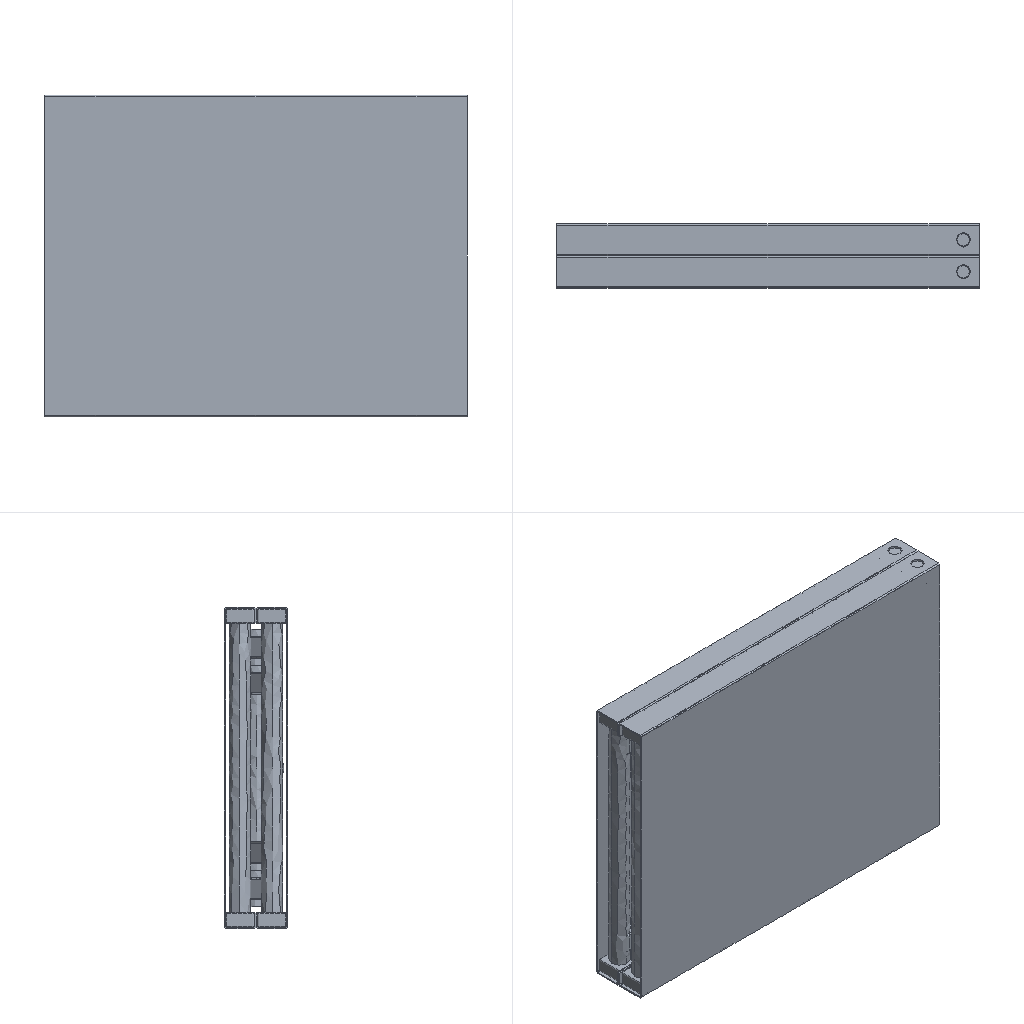Simulation study | abaqus
Set-up summary:
category,name,step,type,value,unit,region
solver,abaqus
solver,version,,,Abaqus/Explicit 2020
units,not stated in the deck,,not stated
analysis,deck,,transient,transient
load_step,Step-1,Step-1,transient
load_step,requested,,,1
mesh,nodes,,,20833
mesh,elements,,,50847
element_type,C3D4,,solid,47612
element_type,C3D8R,,solid,1078
element_type,C3D10M,,solid,2157
load,load commands in deck,,count,3
bc,support commands in deck,,count,8
material,AI,,in results
check,setup vs results,,match,"per instance, exact: element labels, types and connectivity; labels of the nodes the elements use; coordinates not compared"
Abaqus input file, long lists of numbers shortened:
*Heading
** Job name: re-job Model name: Model-1
** Generated by: Abaqus/CAE 2020
*Preprint, echo=NO, model=NO, history=NO, contact=NO
**
** PARTS
**
*Part, name=WORK-1
*Node
      1,   7.262,   37.636,        -192.
      2,  0.8978,          35.,        -192.
** (205 more lines like these left out)
*Element, type=C3D8R
 1,  11,  12,  18,  10,   2,   3,   9,   1
 2,  14,  15,  18,  12,   5,   6,   9,   3
** (86 more lines like these left out)
*Nset, nset=Set-2, generate
   1,  207,    1
*Elset, elset=Set-2, generate
  1,  88,   1
** Section: Section-1
*Solid Section, elset=Set-2, material=AI
,
*End Part
**
*Part, name=WORK-2
*Node
      1,   49.212,   40.328,         -40.
      2,   47.261,   37.408,         -40.
** (872 more lines like these left out)
*Element, type=C3D8R
  1,  69,  42,  43,  56,  31,   4,   5,  18
  2,  43,  44,  70,  56,   5,   6,  32,  18
** (636 more lines like these left out)
*Nset, nset=Set-2, generate
   1,  874,    1
*Elset, elset=Set-2, generate
   1,  638,    1
** Section: Section-1
*Solid Section, elset=Set-2, material=AI
,
*End Part
**
*Part, name=WORK-3
*Node
      1,   221.697,    26.355,         13.5
      2,   221.697,    26.355,        -13.5
** (710 more lines like these left out)
*Element, type=C3D4
   1, 627, 628, 121, 610
   2, 627, 629, 630, 631
** (2272 more lines like these left out)
*Nset, nset=Set-4, generate
   1,  712,    1
*Elset, elset=Set-4, generate
    1,  2274,     1
** Section: Section-1
*Solid Section, elset=Set-4, material=AI
,
*End Part
**
*Part, name=WORK-4
*Node
      1,   220.068,   26.512,        -12.5
      2,   221.266,   38.955,           0.
** (209 more lines like these left out)
*Element, type=C3D4
  1, 191,  70,  71,  78
  2,  45, 192,  38,  37
** (585 more lines like these left out)
*Nset, nset=Set-4, generate
   1,  211,    1
*Elset, elset=Set-4, generate
   1,  587,    1
** Section: Section-1
*Solid Section, elset=Set-4, material=AI
,
*End Part
**
*Part, name=WORK-5
*Node
      1,  -261.84,   59.636,      -220.25
      2,  -268.204,          57.,      -220.25
** (205 more lines like these left out)
*Element, type=C3D8R
 1,  10,  11,  18,  13,   1,   2,   9,   4
 2,  17,  13,  18,  16,   8,   4,   9,   7
** (86 more lines like these left out)
*Nset, nset=Set-2, generate
   1,  207,    1
*Elset, elset=Set-2, generate
  1,  88,   1
** Section: Section-1
*Solid Section, elset=Set-2, material=AI
,
*End Part
**
*Part, name=WORK-6
*Node
      1,   276.364,   59.636,      -220.25
      2,         270.,          57.,      -220.25
** (205 more lines like these left out)
*Element, type=C3D8R
 1,  10,  11,  18,  13,   1,   2,   9,   4
 2,  12,  14,  18,  11,   3,   5,   9,   2
** (86 more lines like these left out)
*Nset, nset=Set-1, generate
   1,  207,    1
*Elset, elset=Set-1, generate
  1,  88,   1
** Section: Section-1
*Solid Section, elset=Set-1, material=AI
,
*End Part
**
*Part, name=WORK-7
*Node
      1,   276.364,   15.636,      -220.25
      2,         270.,          13.,      -220.25
** (205 more lines like these left out)
*Element, type=C3D8R
 1,  18,  11,  12,  14,   9,   2,   3,   5
 2,  10,  11,  18,  13,   1,   2,   9,   4
** (86 more lines like these left out)
*Nset, nset=Set-1, generate
   1,  207,    1
*Elset, elset=Set-1, generate
  1,  88,   1
** Section: Section-1
*Solid Section, elset=Set-1, material=AI
,
*End Part
**
*Part, name=WORK-8
*Node
      1,  -261.84,   15.636,      -220.25
      2,  -268.204,          13.,      -220.25
** (205 more lines like these left out)
*Element, type=C3D8R
 1,  18,  11,  12,  14,   9,   2,   3,   5
 2,  10,  11,  18,  13,   1,   2,   9,   4
** (86 more lines like these left out)
*Nset, nset=Set-1, generate
   1,  207,    1
*Elset, elset=Set-1, generate
  1,  88,   1
** Section: Section-1
*Solid Section, elset=Set-1, material=AI
,
*End Part
**
*Part, name=WORK-9
*Node
      1,  -286.204,          86.,       202.25
      2,  -286.204,          84.,       200.25
** (596 more lines like these left out)
*Element, type=C3D4
   1, 439, 440, 202, 399
   2, 439, 158, 342, 440
** (2114 more lines like these left out)
*Nset, nset=Set-4, generate
   1,  598,    1
*Elset, elset=Set-4, generate
    1,  2116,     1
** Section: Section-1
*Solid Section, elset=Set-4, material=AI
,
*End Part
**
*Part, name=WORK-10
*Node
      1,  -250.204,          86.,      -202.25
      2,  -250.204,          84.,      -200.25
** (3799 more lines like these left out)
*Element, type=C3D10M
   1,  439,  440,  441,  442,  606,  605,  604,  608,  607,  609
   2,  440,  293,  442,  439,  611,  610,  607,  606,  612,  608
** (2155 more lines like these left out)
*Nset, nset=Set-1, generate
    1,  3801,     1
*Elset, elset=Set-1, generate
    1,  2157,     1
** Section: Section-1
*Solid Section, elset=Set-1, material=AI
,
*End Part
**
*Part, name=WORK-11
*Node
      1,         242.,          86.,      -200.25
      2,         242.,          86.,      -219.25
** (1151 more lines like these left out)
*Element, type=C3D4
   1, 1136,   63,   62,  243
   2,    7,   58,   10,   26
** (3214 more lines like these left out)
*Nset, nset=Set-1, generate
    1,  1153,     1
*Elset, elset=Set-1, generate
    1,  3216,     1
** Section: Section-1
*Solid Section, elset=Set-1, material=AI
,
*End Part
**
*Part, name=WORK-12
*Node
      1,  0.08297,   53.967,         142.
      2,  -9.069,   43.185,         142.
** (5124 more lines like these left out)
*Element, type=C3D4
    1, 4402, 1843, 4209, 1844
    2, 1441, 1803, 4209, 1804
** (16189 more lines like these left out)
*Nset, nset=Set-1, generate
    1,  5126,     1
*Elset, elset=Set-1, generate
     1,  16191,      1
** Section: Section-1
*Solid Section, elset=Set-1, material=AI
,
*End Part
**
*Part, name=WORK-13
*Node
      1,  -286.204,          42.,       202.25
      2,  -286.204,          40.,       200.25
** (600 more lines like these left out)
*Element, type=C3D4
   1, 439, 440, 243, 441
   2, 439, 442, 363, 443
** (2147 more lines like these left out)
*Nset, nset=Set-1, generate
   1,  602,    1
*Elset, elset=Set-1, generate
    1,  2149,     1
** Section: Section-1
*Solid Section, elset=Set-1, material=AI
,
*End Part
**
*Part, name=WORK-14
*Node
      1,  -286.204,          42.,      -218.25
      2,  -286.204,          40.,      -220.25
** (600 more lines like these left out)
*Element, type=C3D4
   1, 439, 440, 243, 441
   2, 439, 442, 363, 443
** (2147 more lines like these left out)
*Nset, nset=Set-1, generate
   1,  602,    1
*Elset, elset=Set-1, generate
    1,  2149,     1
** Section: Section-1
*Solid Section, elset=Set-1, material=AI
,
*End Part
**
*Part, name=WORK-15
*Node
      1,  -278.171,   66.815,       200.25
      2,  -258.238,   65.185,       200.25
** (4965 more lines like these left out)
*Element, type=C3D4
    1, 3918, 4688, 4421, 3917
    2, 4689, 3577, 4690, 4348
** (15720 more lines like these left out)
*Nset, nset=Set-1, generate
    1,  4967,     1
*Elset, elset=Set-1, generate
     1,  15722,      1
** Section: Section-1
*Solid Section, elset=Set-1, material=AI
,
*End Part
**
*Part, name=WORK-16
*Node
      1,         242.,           2.,       200.25
      2,         242.,           2.,       219.25
** (1150 more lines like these left out)
*Element, type=C3D4
   1,  388, 1136,   26,  407
   2, 1013,  790,  800,  999
** (3206 more lines like these left out)
*Nset, nset=Set-6, generate
    1,  1152,     1
*Elset, elset=Set-6, generate
    1,  3208,     1
** Section: Section-1
*Solid Section, elset=Set-6, material=AI
,
*End Part
**
**
** ASSEMBLY
**
*Assembly, name=Assembly
**
*Instance, name=WORK-1-1, part=WORK-1
*End Instance
**
*Instance, name=WORK-2-1, part=WORK-2
*End Instance
**
*Instance, name=WORK-3-1, part=WORK-3
*End Instance
**
*Instance, name=WORK-4-1, part=WORK-4
*End Instance
**
*Instance, name=WORK-5-1, part=WORK-5
*End Instance
**
*Instance, name=WORK-6-1, part=WORK-6
*End Instance
**
*Instance, name=WORK-7-1, part=WORK-7
*End Instance
**
*Instance, name=WORK-8-1, part=WORK-8
*End Instance
**
*Instance, name=WORK-9-1, part=WORK-9
*End Instance
**
*Instance, name=WORK-10-1, part=WORK-10
*End Instance
**
*Instance, name=WORK-11-1, part=WORK-11
*End Instance
**
*Instance, name=WORK-12-1, part=WORK-12
*End Instance
**
*Instance, name=WORK-13-1, part=WORK-13
*End Instance
**
*Instance, name=WORK-14-1, part=WORK-14
*End Instance
**
*Instance, name=WORK-15-1, part=WORK-15
*End Instance
**
*Instance, name=WORK-16-1, part=WORK-16
*End Instance
**
*Node
      1,           0.,         100.,           0.
*Nset, nset=Set-1, instance=WORK-16-1
   15,   16,   46,   47,   77,   78,   79,   80,   81,   82,   83,   84,   85,   86,   87,   88
   89,   90,  389,  390,  391,  392,  393,  394,  395,  396,  397,  398,  399,  400,  401,  402
** (20 more lines like these left out)
*Elset, elset=Set-1, instance=WORK-16-1
   19,   34,   38,   48,   50,  234,  236,  244,  245,  247,  248,  250,  252,  253,  254,  256
  260,  265,  266,  270,  272,  273,  274,  278,  279,  284,  290,  299,  308,  309,  313,  315
** (37 more lines like these left out)
*Nset, nset=Set-2, instance=WORK-11-1
   15,   16,   46,   47,   77,   78,   79,   80,   81,   82,   83,   84,   85,   86,   87,   88
   89,   90,  389,  390,  391,  392,  393,  394,  395,  396,  397,  398,  399,  400,  401,  402
** (20 more lines like these left out)
*Elset, elset=Set-2, instance=WORK-11-1
    7,    8,   60,   64,   67,   82,   94,  146,  261,  263,  266,  267,  276,  278,  279,  283
  284,  285,  287,  292,  297,  298,  302,  304,  310,  314,  315,  320,  322,  333,  336,  339
** (37 more lines like these left out)
*Nset, nset=Set-4
 1,
*Nset, nset=Set-5, instance=WORK-7-1
   1,   2,   3,   4,   5,   6,   7,   8,   9, 199, 200, 201, 202, 203, 204, 205
 206, 207
*Nset, nset=Set-5, instance=WORK-8-1
   1,   2,   3,   4,   5,   6,   7,   8,   9, 199, 200, 201, 202, 203, 204, 205
 206, 207
*Elset, elset=Set-5, instance=WORK-7-1
  1,  2,  3,  4, 85, 86, 87, 88
*Elset, elset=Set-5, instance=WORK-8-1
  1,  2,  3,  4, 85, 86, 87, 88
*Nset, nset=Set-6
 1,
*Nset, nset=Set-7, instance=WORK-7-1
   1,   2,   3,   4,   5,   6,   7,   8,   9, 199, 200, 201, 202, 203, 204, 205
 206, 207
*Elset, elset=Set-7, instance=WORK-7-1
  1,  2,  3,  4, 85, 86, 87, 88
*Nset, nset=Set-8, instance=WORK-8-1
   1,   2,   3,   4,   5,   6,   7,   8,   9, 199, 200, 201, 202, 203, 204, 205
 206, 207
*Elset, elset=Set-8, instance=WORK-8-1
  1,  2,  3,  4, 85, 86, 87, 88
*Nset, nset=Set-9, instance=WORK-5-1
   1,   2,   3,   4,   5,   6,   7,   8,   9, 199, 200, 201, 202, 203, 204, 205
 206, 207
*Nset, nset=Set-9, instance=WORK-8-1
   1,   2,   3,   4,   5,   6,   7,   8,   9, 199, 200, 201, 202, 203, 204, 205
 206, 207
*Elset, elset=Set-9, instance=WORK-5-1
  1,  2,  3,  4, 85, 86, 87, 88
*Elset, elset=Set-9, instance=WORK-8-1
  1,  2,  3,  4, 85, 86, 87, 88
*Nset, nset=Set-10, instance=WORK-8-1
   1,   2,   3,   4,   5,   6,   7,   8,   9, 199, 200, 201, 202, 203, 204, 205
 206, 207
*Elset, elset=Set-10, instance=WORK-8-1
  1,  2,  3,  4, 85, 86, 87, 88
*Nset, nset=m_Set-3
 1,
*Elset, elset=_m_Surf-1_S2, internal, instance=WORK-5-1, generate
 1,  4,  1
*Surface, type=ELEMENT, name=m_Surf-1
_m_Surf-1_S2, S2
*Elset, elset=_m_Surf-3_S1, internal, instance=WORK-5-1, generate
 85,  88,   1
*Surface, type=ELEMENT, name=m_Surf-3
_m_Surf-3_S1, S1
*Elset, elset=_m_Surf-5_S1, internal, instance=WORK-8-1, generate
 85,  88,   1
*Surface, type=ELEMENT, name=m_Surf-5
_m_Surf-5_S1, S1
*Elset, elset=_m_Surf-7_S2, internal, instance=WORK-8-1, generate
 1,  4,  1
*Surface, type=ELEMENT, name=m_Surf-7
_m_Surf-7_S2, S2
*Elset, elset=_m_Surf-9_S2, internal, instance=WORK-1-1, generate
 1,  4,  1
*Surface, type=ELEMENT, name=m_Surf-9
_m_Surf-9_S2, S2
*Elset, elset=_m_Surf-11_S1, internal, instance=WORK-1-1, generate
 85,  88,   1
*Surface, type=ELEMENT, name=m_Surf-11
_m_Surf-11_S1, S1
*Elset, elset=_m_Surf-13_S1, internal, instance=WORK-2-1, generate
 610,  638,    1
*Surface, type=ELEMENT, name=m_Surf-13
_m_Surf-13_S1, S1
*Elset, elset=_m_Surf-15_S2, internal, instance=WORK-2-1, generate
  1,  29,   1
*Surface, type=ELEMENT, name=m_Surf-15
_m_Surf-15_S2, S2
*Elset, elset=_m_Surf-17_S2, internal, instance=WORK-7-1, generate
 1,  4,  1
*Surface, type=ELEMENT, name=m_Surf-17
_m_Surf-17_S2, S2
*Elset, elset=_m_Surf-19_S1, internal, instance=WORK-7-1, generate
 85,  88,   1
*Surface, type=ELEMENT, name=m_Surf-19
_m_Surf-19_S1, S1
*Elset, elset=_m_Surf-22_S3, internal, instance=WORK-11-1
 1265, 1636, 1824, 1874, 1936, 1947, 1950, 1954, 1958, 1963, 1969, 1971, 1973, 1976, 1979, 1980
 1982, 1983, 1986, 1988, 1991, 1998, 2003, 2005, 2006, 2008, 2025, 2251, 2301, 2337, 2634, 3199
*Elset, elset=_m_Surf-22_S1, internal, instance=WORK-11-1
 1934,
*Elset, elset=_m_Surf-22_S4, internal, instance=WORK-11-1
 1941, 2218, 2557
*Surface, type=ELEMENT, name=m_Surf-22
_m_Surf-22_S3, S3
_m_Surf-22_S1, S1
_m_Surf-22_S4, S4
*Elset, elset=_s_Surf-1_S2, internal, instance=WORK-10-1
  140, 1162, 1179, 1284, 1319
*Elset, elset=_s_Surf-1_S3, internal, instance=WORK-10-1
  228,  253,  281,  404,  415,  419,  563,  667,  684,  703,  736,  778,  783,  803,  806,  815
  821,  823,  883,  906,  940,  942, 1083, 1095, 1104, 1120, 1129, 1143, 1148, 1152, 1153, 1157
** (3 more lines like these left out)
*Elset, elset=_s_Surf-1_S4, internal, instance=WORK-10-1
  521,  537,  973, 1043, 1115, 1300, 1361
*Elset, elset=_s_Surf-1_S1, internal, instance=WORK-10-1
 1348,
*Surface, type=ELEMENT, name=s_Surf-1
_s_Surf-1_S2, S2
_s_Surf-1_S3, S3
_s_Surf-1_S4, S4
_s_Surf-1_S1, S1
*Elset, elset=_s_Surf-3_S3, internal, instance=WORK-9-1
   10,   26,  116,  277,  444,  455,  678,  700,  809,  827,  837,  877,  880,  938,  942,  944
  977, 1008, 1017, 1034, 1068, 1075, 1078, 1080, 1081, 1119, 1123, 1127, 1138, 1173, 1179, 1184
** (3 more lines like these left out)
*Elset, elset=_s_Surf-3_S1, internal, instance=WORK-9-1
  121, 1140, 1607, 2045
*Elset, elset=_s_Surf-3_S4, internal, instance=WORK-9-1
  197,  202, 1033, 1085
*Elset, elset=_s_Surf-3_S2, internal, instance=WORK-9-1
  497, 1020, 1159, 1164, 1185
*Surface, type=ELEMENT, name=s_Surf-3
_s_Surf-3_S3, S3
_s_Surf-3_S1, S1
_s_Surf-3_S4, S4
_s_Surf-3_S2, S2
*Elset, elset=_s_Surf-5_S3, internal, instance=WORK-13-1
  114,  116,  234,  305,  308,  407,  515,  541,  561,  574,  582,  606,  619,  655,  738,  879
  883,  931,  933,  939,  945,  973,  996, 1008, 1051, 1053, 1055, 1062, 1078, 1087, 1122, 1135
** (3 more lines like these left out)
*Elset, elset=_s_Surf-5_S2, internal, instance=WORK-13-1
  224, 1098, 1177, 1548
*Elset, elset=_s_Surf-5_S4, internal, instance=WORK-13-1
  337, 1329, 1337, 1539, 1597
*Surface, type=ELEMENT, name=s_Surf-5
_s_Surf-5_S3, S3
_s_Surf-5_S2, S2
_s_Surf-5_S4, S4
*Elset, elset=_s_Surf-7_S4, internal, instance=WORK-14-1
 147, 353, 551, 868, 957
*Elset, elset=_s_Surf-7_S2, internal, instance=WORK-14-1
  189,  217,  907, 1308, 1665, 1867, 2009
*Elset, elset=_s_Surf-7_S3, internal, instance=WORK-14-1
  253,  360,  508,  694,  719,  789,  902,  910,  911,  960,  966,  989, 1018, 1106, 1118, 1227
 1266, 1313, 1447, 1468, 1469, 1478, 1490, 1517, 1531, 1672, 1676, 1736, 1745, 1795, 1808, 1813
** (3 more lines like these left out)
*Elset, elset=_s_Surf-7_S1, internal, instance=WORK-14-1
 1152, 1233, 1278
*Surface, type=ELEMENT, name=s_Surf-7
_s_Surf-7_S4, S4
_s_Surf-7_S2, S2
_s_Surf-7_S3, S3
_s_Surf-7_S1, S1
*Elset, elset=_s_Surf-9_S3, internal, instance=WORK-15-1
   19,   20, 4468, 8664, 8738, 9003
*Elset, elset=_s_Surf-9_S4, internal, instance=WORK-15-1
   917,  8114,  8551,  8679,  8687,  8734,  9651, 12450
*Elset, elset=_s_Surf-9_S2, internal, instance=WORK-15-1
  7329,  8970, 11381, 14219
*Elset, elset=_s_Surf-9_S1, internal, instance=WORK-15-1
 9655,
*Surface, type=ELEMENT, name=s_Surf-9
_s_Surf-9_S3, S3
_s_Surf-9_S4, S4
_s_Surf-9_S2, S2
_s_Surf-9_S1, S1
*Elset, elset=_s_Surf-11_S3, internal, instance=WORK-15-1
   204,  1697,  6734,  7453,  8763,  8825,  8840,  9844,  9986,  9988,  9997,  9998, 10074, 10289
*Elset, elset=_s_Surf-11_S4, internal, instance=WORK-15-1
   654,  1522,  9991, 10290
*Elset, elset=_s_Surf-11_S1, internal, instance=WORK-15-1
 12418,
*Surface, type=ELEMENT, name=s_Surf-11
_s_Surf-11_S3, S3
_s_Surf-11_S4, S4
_s_Surf-11_S1, S1
*Elset, elset=_s_Surf-13_S3, internal, instance=WORK-12-1
    39,   233,   457,  1169,  1170,  9256,  9276,  9284,  9342,  9351,  9464,  9510,  9515,  9607,  9940, 11445
 11625,
*Elset, elset=_s_Surf-13_S2, internal, instance=WORK-12-1
 440,
*Elset, elset=_s_Surf-13_S1, internal, instance=WORK-12-1
  442, 9272
*Elset, elset=_s_Surf-13_S4, internal, instance=WORK-12-1
  1168,  9617,  9901, 11439
*Surface, type=ELEMENT, name=s_Surf-13
_s_Surf-13_S3, S3
_s_Surf-13_S2, S2
_s_Surf-13_S4, S4
_s_Surf-13_S1, S1
*Elset, elset=_s_Surf-15_S4, internal, instance=WORK-12-1
    30,  7769,  7956, 12024, 15156
*Elset, elset=_s_Surf-15_S3, internal, instance=WORK-12-1
    77,   187,  1341,  3155,  5025,  5391,  6906,  6913,  7975, 10011, 12041, 15675, 15787, 15804, 15808, 15815
 15823,
*Elset, elset=_s_Surf-15_S2, internal, instance=WORK-12-1
 5422,
*Elset, elset=_s_Surf-15_S1, internal, instance=WORK-12-1
 15677,
*Surface, type=ELEMENT, name=s_Surf-15
_s_Surf-15_S4, S4
_s_Surf-15_S3, S3
_s_Surf-15_S2, S2
_s_Surf-15_S1, S1
*Elset, elset=_s_Surf-17_S4, internal, instance=WORK-16-1
   36,  121,  125,  128,  145,  146,  147,  148,  150,  167,  170,  171,  173,  179,  187,  208
  209,  217,  221,  224,  846, 1879, 1990, 2024, 2135, 2240, 2241, 2579, 2637, 2670, 2681, 2712
** (1 more lines like these left out)
*Elset, elset=_s_Surf-17_S3, internal, instance=WORK-16-1
   51,   55,   76,  158,  169,  175,  211,  769, 2086, 2108, 2157, 2160, 2552
*Elset, elset=_s_Surf-17_S1, internal, instance=WORK-16-1
   68,  116,  186,  188,  191,  214,  996, 1421, 1827, 2286, 2642, 2690, 2727, 2981, 2986, 2987
 2997, 3037
*Elset, elset=_s_Surf-17_S2, internal, instance=WORK-16-1
   89,  124,  140,  168,  184,  192,  199,  218,  222,  267,  351,  480, 1050, 1137, 2080, 2536
 2555, 2583, 2892, 2896, 2897, 2954, 2959
*Surface, type=ELEMENT, name=s_Surf-17
_s_Surf-17_S4, S4
_s_Surf-17_S3, S3
_s_Surf-17_S2, S2
_s_Surf-17_S1, S1
*Elset, elset=_s_Surf-19_S3, internal, instance=WORK-16-1
   21,   74,   75,  924, 1760, 1906, 1979, 2199
*Elset, elset=_s_Surf-19_S2, internal, instance=WORK-16-1
  511, 1047, 1707, 1711, 1715, 1719, 1723, 1728, 1751, 1828, 1851, 1893, 1897, 1957, 1959, 1971
 1974, 2015, 2151, 2190, 2360, 2384
*Elset, elset=_s_Surf-19_S4, internal, instance=WORK-16-1
  607, 1714, 1741, 1782, 1792, 1794, 1802, 1818, 1835, 1853, 1868, 1875, 1907, 1910, 1922, 1926
 1949, 1953, 1996, 2019, 2025, 2105, 2269, 2296, 2301, 2303, 2308, 2317, 2321, 2325, 3136
*Elset, elset=_s_Surf-19_S1, internal, instance=WORK-16-1
 1708, 1709, 1718, 1722, 1732, 1735, 1742, 1744, 1750, 1769, 1780, 1781, 1785, 1805, 1809, 1813
 1816, 1819, 1837, 1925, 1928, 1938, 1972, 1993, 2014, 2282, 2351, 2387, 2851
*Surface, type=ELEMENT, name=s_Surf-19
_s_Surf-19_S3, S3
_s_Surf-19_S2, S2
_s_Surf-19_S4, S4
_s_Surf-19_S1, S1
*Elset, elset=_s_Surf-21_S3, internal, instance=WORK-11-1
    7,    8,  298,  302,  310,  320,  322,  339,  409,  512,  548,  563,  621,  648,  670,  699
  740,  760,  786,  845,  847,  850,  854,  896,  924,  985, 1007, 1041, 1070, 1074, 1110, 1133
** (3 more lines like these left out)
*Elset, elset=_s_Surf-21_S2, internal, instance=WORK-11-1
   60,   67,   82,   94,  146,  261,  263,  278,  285,  287,  292,  297,  314,  341,  349,  350
  357,  362,  365,  371,  372,  374,  381,  383,  388,  399,  402,  419,  423,  427,  433,  439
** (12 more lines like these left out)
*Elset, elset=_s_Surf-21_S4, internal, instance=WORK-11-1
   64,  266,  283,  304,  315,  333,  354,  360,  369,  375,  380,  384,  385,  407,  443,  477
  487,  493,  518,  524,  532,  547,  564,  586,  590,  627,  654,  669,  678,  679,  681,  707
** (7 more lines like these left out)
*Elset, elset=_s_Surf-21_S1, internal, instance=WORK-11-1
  267,  276,  279,  284,  336,  344,  364,  391,  397,  404,  429,  448,  459,  467,  474,  508
  509,  515,  520,  535,  541,  574,  583,  594,  615,  622,  624,  625,  634,  693,  708,  709
** (9 more lines like these left out)
*Surface, type=ELEMENT, name=s_Surf-21
_s_Surf-21_S3, S3
_s_Surf-21_S2, S2
_s_Surf-21_S4, S4
_s_Surf-21_S1, S1
*Elset, elset=_s_Surf-22_S1, internal, instance=WORK-5-1, generate
 85,  88,   1
*Elset, elset=_s_Surf-22_S1, internal, instance=WORK-6-1, generate
 85,  88,   1
*Elset, elset=_s_Surf-22_S2, internal, instance=WORK-5-1, generate
 1,  4,  1
*Elset, elset=_s_Surf-22_S2, internal, instance=WORK-6-1, generate
 1,  4,  1
*Surface, type=ELEMENT, name=s_Surf-22
_s_Surf-22_S1, S1
_s_Surf-22_S2, S2
*Elset, elset=_s_Surf-24_S1, internal, instance=WORK-6-1, generate
 85,  88,   1
*Elset, elset=_s_Surf-24_S2, internal, instance=WORK-6-1, generate
 1,  4,  1
*Surface, type=ELEMENT, name=s_Surf-24
_s_Surf-24_S1, S1
_s_Surf-24_S2, S2
** Constraint: Constraint-5
*Tie, name=Constraint-5, adjust=yes
s_Surf-9, m_Surf-9
** Constraint: Constraint-6
*Tie, name=Constraint-6, adjust=yes
s_Surf-11, m_Surf-11
** Constraint: Constraint-7
*Tie, name=Constraint-7, adjust=yes
s_Surf-13, m_Surf-13
** Constraint: Constraint-8
*Tie, name=Constraint-8, adjust=yes
s_Surf-15, m_Surf-15
** Constraint: v
*Coupling, constraint name=v, ref node=m_Set-3, surface=s_Surf-21
*Kinematic
*End Assembly
**
** MATERIALS
**
*Material, name=AI
*Density
 2.8e-09,
*Elastic
70000., 0.33
**
** INTERACTION PROPERTIES
**
*Surface Interaction, name=IntProp-1
*Friction
 0.1,
*Surface Behavior, pressure-overclosure=HARD
** ----------------------------------------------------------------
**
** STEP: Step-1
**
*Step, name=Step-1, nlgeom=YES
*Dynamic, Explicit
, 4.5
*Bulk Viscosity
0.06, 1.2
** Mass Scaling: Semi-Automatic
**               Whole Model
*Fixed Mass Scaling, dt=1e-05, type=below min
**
** BOUNDARY CONDITIONS
**
** Name: BC-1 Type: 对称/反对称/完全固定
*Boundary
Set-1, ENCASTRE
** Name: BC-3 Type: 位移/转角
*Boundary
Set-7, 3, 3
** Name: v Type: velocity/angular velocity
*Boundary, type=VELOCITY
Set-4, 1, 1
Set-4, 2, 2, 50.
Set-4, 3, 3
Set-4, 4, 4
Set-4, 5, 5
Set-4, 6, 6
**
** LOADS
**
** Name: Load-1   Type: Gravity
*Dload
, GRAV, 9800., 0., -1., 0.
** Name: Load-2   Type: Concentrated force
*Cload
Set-6, 2, -960.
**
** INTERACTIONS
**
** Interaction: Int-1
*Contact, op=NEW
*Contact Inclusions, ALL EXTERIOR
*Contact Property Assignment
 ,  , IntProp-1
**
** OUTPUT REQUESTS
**
*Restart, write, number interval=1, time marks=NO
**
** FIELD OUTPUT: F-Output-1
**
*Output, field, number interval=200
*Node Output
A, RF, U, V
*Element Output, directions=YES
E, LE, MISES, PE, PEEQ, PEEQVAVG, PEVAVG, S, SVAVG
*Contact Output
CFORCE, CSTRESS
**
** HISTORY OUTPUT: H-Output-1
**
*Output, history, variable=PRESELECT
*End Step
Results summary:
result,step,Step-1,completed,increments=496847 time=4.5/4.5
result,analysis,,,transient
result,last_loadstep,,,1
result,primary field,,,U
result,reaction total,,FX,610.739,model units
result,reaction total,,FY,973.762,model units
result,reaction total,,FZ,-804.503,model units